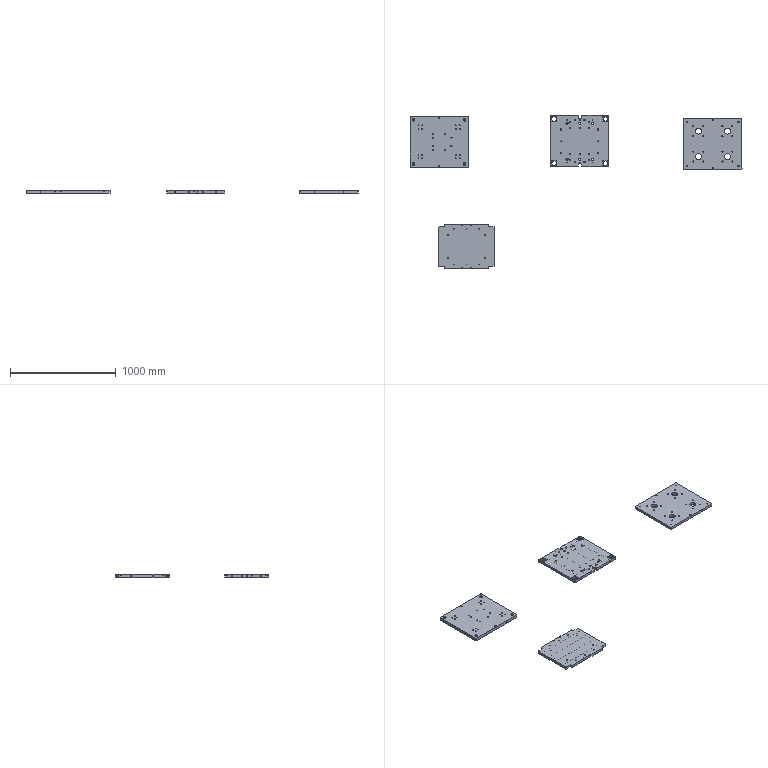NC program | Mastercam | posted with a generic post | part box 3140 x 1452 x 30 mm
Lines 2204 to 3077 of 22248:
N2200 T16 M6
N2210 G0 G90 G17 G54 X-237.285 Y214.441 A0. S6000 M3
N2220 G43 H16 Z50. M8
N2230 Z3.3
N2240 G1 Z.5 F600.
N2250 G3 X-242. Y216.2 Z.437 I-4.715 J-5.441 F3000.
N2260 X-249.2 Y209. Z.299 I0. J-7.2
N2270 X-242. Y201.8 Z.161 I7.2 J0.
N2280 X-234.8 Y209. Z.023 I0. J7.2
N2290 X-242. Y216.2 Z-.116 I-7.2 J0.
N2300 X-249.2 Y209. Z-.254 I0. J-7.2
N2310 X-242. Y201.8 Z-.392 I7.2 J0.
N2320 X-234.8 Y209. Z-.53 I0. J7.2
N2330 X-242. Y216.2 Z-.668 I-7.2 J0.
N2340 X-249.2 Y209. Z-.806 I0. J-7.2
N2350 X-242. Y201.8 Z-.945 I7.2 J0.
N2360 X-234.8 Y209. Z-1.083 I0. J7.2
N2370 X-242. Y216.2 Z-1.221 I-7.2 J0.
N2380 X-249.2 Y209. Z-1.359 I0. J-7.2
N2390 X-242. Y201.8 Z-1.497 I7.2 J0.
N2400 X-234.8 Y209. Z-1.636 I0. J7.2
N2410 X-242. Y216.2 Z-1.774 I-7.2 J0.
N2420 X-249.2 Y209. Z-1.912 I0. J-7.2
N2430 X-242. Y201.8 Z-2.05 I7.2 J0.
N2440 X-234.8 Y209. Z-2.188 I0. J7.2
N2450 X-242. Y216.2 Z-2.326 I-7.2 J0.
N2460 X-249.2 Y209. Z-2.465 I0. J-7.2
N2470 X-242. Y201.8 Z-2.603 I7.2 J0.
N2480 X-234.8 Y209. Z-2.741 I0. J7.2
N2490 X-242. Y216.2 Z-2.879 I-7.2 J0.
N2500 X-249.2 Y209. Z-3.017 I0. J-7.2
N2510 X-242. Y201.8 Z-3.156 I7.2 J0.
N2520 X-234.8 Y209. Z-3.294 I0. J7.2
N2530 X-242. Y216.2 Z-3.432 I-7.2 J0.
N2540 X-249.2 Y209. Z-3.57 I0. J-7.2
N2550 X-242. Y201.8 Z-3.708 I7.2 J0.
N2560 X-234.8 Y209. Z-3.846 I0. J7.2
N2570 X-242. Y216.2 Z-3.985 I-7.2 J0.
N2580 X-249.2 Y209. Z-4.123 I0. J-7.2
N2590 X-242. Y201.8 Z-4.261 I7.2 J0.
N2600 X-234.8 Y209. Z-4.399 I0. J7.2
N2610 X-242. Y216.2 Z-4.537 I-7.2 J0.
N2620 X-249.2 Y209. Z-4.676 I0. J-7.2
N2630 X-242. Y201.8 Z-4.814 I7.2 J0.
N2640 X-234.8 Y209. Z-4.952 I0. J7.2
N2650 X-242. Y216.2 Z-5.09 I-7.2 J0.
N2660 X-249.2 Y209. Z-5.228 I0. J-7.2
N2670 X-242. Y201.8 Z-5.366 I7.2 J0.
N2680 X-234.8 Y209. Z-5.505 I0. J7.2
N2690 X-242. Y216.2 Z-5.643 I-7.2 J0.
N2700 X-249.2 Y209. Z-5.781 I0. J-7.2
N2710 X-242. Y201.8 Z-5.919 I7.2 J0.
N2720 X-234.8 Y209. Z-6.057 I0. J7.2
N2730 X-242. Y216.2 Z-6.196 I-7.2 J0.
N2740 X-249.2 Y209. Z-6.334 I0. J-7.2
N2750 X-242. Y201.8 Z-6.472 I7.2 J0.
N2760 X-234.8 Y209. Z-6.61 I0. J7.2
N2770 X-242. Y216.2 Z-6.748 I-7.2 J0.
N2780 X-249.2 Y209. Z-6.886 I0. J-7.2
N2790 X-242. Y201.8 Z-7.025 I7.2 J0.
N2800 X-234.8 Y209. Z-7.163 I0. J7.2
N2810 X-242. Y216.2 Z-7.301 I-7.2 J0.
N2820 X-249.2 Y209. Z-7.439 I0. J-7.2
N2830 X-242. Y201.8 Z-7.577 I7.2 J0.
N2840 X-234.8 Y209. Z-7.716 I0. J7.2
N2850 X-242. Y216.2 Z-7.854 I-7.2 J0.
N2860 X-249.2 Y209. Z-7.992 I0. J-7.2
N2870 X-242. Y201.8 Z-8.13 I7.2 J0.
N2880 X-234.8 Y209. Z-8.268 I0. J7.2
N2890 X-242. Y216.2 Z-8.406 I-7.2 J0.
N2900 X-249.2 Y209. Z-8.545 I0. J-7.2
N2910 X-242. Y201.8 Z-8.683 I7.2 J0.
N2920 X-234.8 Y209. Z-8.821 I0. J7.2
N2930 X-242. Y216.2 Z-8.959 I-7.2 J0.
N2940 X-249.2 Y209. Z-9.097 I0. J-7.2
N2950 X-242. Y201.8 Z-9.236 I7.2 J0.
N2960 X-234.8 Y209. Z-9.374 I0. J7.2
N2970 X-242. Y216.2 Z-9.512 I-7.2 J0.
N2980 X-249.2 Y209. Z-9.65 I0. J-7.2
N2990 X-242. Y201.8 Z-9.788 I7.2 J0.
N3000 X-234.8 Y209. Z-9.926 I0. J7.2
N3010 X-242. Y216.2 Z-10.065 I-7.2 J0.
N3020 X-249.2 Y209. Z-10.203 I0. J-7.2
N3030 X-242. Y201.8 Z-10.341 I7.2 J0.
N3040 X-234.8 Y209. Z-10.479 I0. J7.2
N3050 X-242. Y216.2 Z-10.617 I-7.2 J0.
N3060 X-249.2 Y209. Z-10.756 I0. J-7.2
N3070 X-242. Y201.8 Z-10.894 I7.2 J0.
N3080 X-234.8 Y209. Z-11.032 I0. J7.2
N3090 X-242. Y216.2 Z-11.17 I-7.2 J0.
N3100 X-249.2 Y209. Z-11.308 I0. J-7.2
N3110 X-242. Y201.8 Z-11.446 I7.2 J0.
N3120 X-234.8 Y209. Z-11.585 I0. J7.2
N3130 X-242. Y216.2 Z-11.723 I-7.2 J0.
N3140 X-249.2 Y209. Z-11.861 I0. J-7.2
N3150 X-242. Y201.8 Z-11.999 I7.2 J0.
N3160 X-234.8 Y209. Z-12.137 I0. J7.2
N3170 X-242. Y216.2 Z-12.275 I-7.2 J0.
N3180 X-249.2 Y209. Z-12.414 I0. J-7.2
N3190 X-242. Y201.8 Z-12.552 I7.2 J0.
N3200 X-234.8 Y209. Z-12.69 I0. J7.2
N3210 X-242. Y216.2 Z-12.828 I-7.2 J0.
N3220 X-249.2 Y209. Z-12.966 I0. J-7.2
N3230 X-242. Y201.8 Z-13.105 I7.2 J0.
N3240 X-234.8 Y209. Z-13.243 I0. J7.2
N3250 X-242. Y216.2 Z-13.381 I-7.2 J0.
N3260 X-249.2 Y209. Z-13.519 I0. J-7.2
N3270 X-242. Y201.8 Z-13.657 I7.2 J0.
N3280 X-234.8 Y209. Z-13.795 I0. J7.2
N3290 X-242. Y216.2 Z-13.934 I-7.2 J0.
N3300 X-249.2 Y209. Z-14.072 I0. J-7.2
N3310 X-242. Y201.8 Z-14.21 I7.2 J0.
N3320 X-234.8 Y209. Z-14.348 I0. J7.2
N3330 X-242. Y216.2 Z-14.486 I-7.2 J0.
N3340 X-249.2 Y209. Z-14.625 I0. J-7.2
N3350 X-242. Y201.8 Z-14.763 I7.2 J0.
N3360 X-234.8 Y209. Z-14.901 I0. J7.2
N3370 X-242. Y216.2 Z-15.039 I-7.2 J0.
N3380 X-249.2 Y209. Z-15.177 I0. J-7.2
N3390 X-242. Y201.8 Z-15.315 I7.2 J0.
N3400 X-234.8 Y209. Z-15.454 I0. J7.2
N3410 X-242. Y216.2 Z-15.592 I-7.2 J0.
N3420 X-249.2 Y209. Z-15.73 I0. J-7.2
N3430 X-242. Y201.8 Z-15.868 I7.2 J0.
N3440 X-234.8 Y209. Z-16.006 I0. J7.2
N3450 X-242. Y216.2 Z-16.145 I-7.2 J0.
N3460 X-249.2 Y209. Z-16.283 I0. J-7.2
N3470 X-242. Y201.8 Z-16.421 I7.2 J0.
N3480 X-234.8 Y209. Z-16.559 I0. J7.2
N3490 X-242. Y216.2 Z-16.697 I-7.2 J0.
N3500 X-249.2 Y209. Z-16.835 I0. J-7.2
N3510 X-242. Y201.8 Z-16.974 I7.2 J0.
N3520 X-234.8 Y209. Z-17.112 I0. J7.2
N3530 X-242. Y216.2 Z-17.25 I-7.2 J0.
N3540 X-249.2 Y209. Z-17.388 I0. J-7.2
N3550 X-242. Y201.8 Z-17.526 I7.2 J0.
N3560 X-234.8 Y209. Z-17.665 I0. J7.2
N3570 X-242. Y216.2 Z-17.803 I-7.2 J0.
N3580 X-249.2 Y209. Z-17.941 I0. J-7.2
N3590 X-242. Y201.8 Z-18.079 I7.2 J0.
N3600 X-234.8 Y209. Z-18.217 I0. J7.2
N3610 X-242. Y216.2 Z-18.355 I-7.2 J0.
N3620 X-249.2 Y209. Z-18.494 I0. J-7.2
N3630 X-242. Y201.8 Z-18.632 I7.2 J0.
N3640 X-234.8 Y209. Z-18.77 I0. J7.2
N3650 X-242. Y216.2 Z-18.908 I-7.2 J0.
N3660 X-249.2 Y209. Z-19.046 I0. J-7.2
N3670 X-242. Y201.8 Z-19.185 I7.2 J0.
N3680 X-234.8 Y209. Z-19.323 I0. J7.2
N3690 X-242. Y216.2 Z-19.461 I-7.2 J0.
N3700 X-249.2 Y209. Z-19.599 I0. J-7.2
N3710 X-242. Y201.8 Z-19.737 I7.2 J0.
N3720 X-234.8 Y209. Z-19.875 I0. J7.2
N3730 X-242. Y216.2 Z-20.014 I-7.2 J0.
N3740 X-249.2 Y209. Z-20.152 I0. J-7.2
N3750 X-242. Y201.8 Z-20.29 I7.2 J0.
N3760 X-234.8 Y209. Z-20.428 I0. J7.2
N3770 X-242. Y216.2 Z-20.566 I-7.2 J0.
N3780 X-249.2 Y209. Z-20.705 I0. J-7.2
N3790 X-242. Y201.8 Z-20.843 I7.2 J0.
N3800 X-234.8 Y209. Z-20.981 I0. J7.2
N3810 X-242. Y216.2 Z-21.119 I-7.2 J0.
N3820 X-249.2 Y209. Z-21.257 I0. J-7.2
N3830 X-242. Y201.8 Z-21.395 I7.2 J0.
N3840 X-234.8 Y209. Z-21.534 I0. J7.2
N3850 X-242. Y216.2 Z-21.672 I-7.2 J0.
N3860 X-249.2 Y209. Z-21.81 I0. J-7.2
N3870 X-242. Y201.8 Z-21.948 I7.2 J0.
N3880 X-234.8 Y209. Z-22.086 I0. J7.2
N3890 X-242. Y216.2 Z-22.225 I-7.2 J0.
N3900 X-249.2 Y209. Z-22.363 I0. J-7.2
N3910 X-242. Y201.8 Z-22.501 I7.2 J0.
N3920 X-234.8 Y209. Z-22.639 I0. J7.2
N3930 X-242. Y216.2 Z-22.777 I-7.2 J0.
N3940 X-249.2 Y209. Z-22.915 I0. J-7.2
N3950 X-242. Y201.8 Z-23.054 I7.2 J0.
N3960 X-234.8 Y209. Z-23.192 I0. J7.2
N3970 X-242. Y216.2 Z-23.33 I-7.2 J0.
N3980 X-249.2 Y209. Z-23.468 I0. J-7.2
N3990 X-242. Y201.8 Z-23.606 I7.2 J0.
N4000 X-234.8 Y209. Z-23.745 I0. J7.2
N4010 X-242. Y216.2 Z-23.883 I-7.2 J0.
N4020 X-249.2 Y209. Z-24.021 I0. J-7.2
N4030 X-242. Y201.8 Z-24.159 I7.2 J0.
N4040 X-234.8 Y209. Z-24.297 I0. J7.2
N4050 X-242. Y216.2 Z-24.435 I-7.2 J0.
N4060 X-249.2 Y209. Z-24.574 I0. J-7.2
N4070 X-242. Y201.8 Z-24.712 I7.2 J0.
N4080 X-234.8 Y209. Z-24.85 I0. J7.2
N4090 X-242. Y216.2 I-7.2 J0.
N4100 X-249.2 Y209. I0. J-7.2
N4110 X-242. Y201.8 I7.2 J0.
N4120 X-234.8 Y209. I0. J7.2
N4130 G1 X-234.788 Y209.214
N4140 X-234.783 Y209.401
N4150 X-234.789 Y209.629
N4160 X-234.807 Y209.881
N4170 X-234.839 Y210.147
N4180 X-234.883 Y210.42
N4190 X-234.94 Y210.697
N4200 X-235.01 Y210.975
N4210 X-235.091 Y211.252
N4220 X-235.184 Y211.527
N4230 X-235.289 Y211.798
N4240 X-235.404 Y212.066
N4250 X-235.531 Y212.329
N4260 X-235.668 Y212.587
N4270 X-235.815 Y212.839
N4280 X-235.973 Y213.085
N4290 X-236.14 Y213.325
N4300 X-236.317 Y213.558
N4310 X-236.503 Y213.783
N4320 X-236.698 Y214.001
N4330 X-236.901 Y214.211
N4340 X-237.113 Y214.412
N4350 X-237.332 Y214.605
N4360 X-237.559 Y214.789
N4370 X-237.793 Y214.964
N4380 X-238.034 Y215.129
N4390 X-238.281 Y215.284
N4400 X-238.535 Y215.429
N4410 X-238.793 Y215.564
N4420 X-239.057 Y215.689
N4430 X-239.326 Y215.803
N4440 X-239.599 Y215.906
N4450 X-239.876 Y215.998
N4460 X-240.157 Y216.079
N4470 X-240.44 Y216.149
N4480 X-240.726 Y216.207
N4490 X-241.014 Y216.254
N4500 X-241.303 Y216.289
N4510 X-241.594 Y216.313
N4520 X-241.886 Y216.325
N4530 X-242.178 Y216.326
N4540 X-242.469 Y216.315
N4550 X-242.76 Y216.292
N4560 X-243.05 Y216.258
N4570 X-243.338 Y216.213
N4580 X-243.624 Y216.156
N4590 X-243.908 Y216.087
N4600 X-244.188 Y216.008
N4610 X-244.466 Y215.917
N4620 X-244.739 Y215.815
N4630 X-245.009 Y215.703
N4640 X-245.273 Y215.58
N4650 X-245.533 Y215.446
N4660 X-245.787 Y215.303
N4670 X-246.035 Y215.149
N4680 X-246.277 Y214.986
N4690 X-246.512 Y214.813
N4700 X-246.74 Y214.631
N4710 X-246.961 Y214.44
N4720 X-247.174 Y214.24
N4730 X-247.379 Y214.032
N4740 X-247.576 Y213.816
N4750 X-247.763 Y213.593
N4760 X-247.942 Y213.362
N4770 X-248.112 Y213.125
N4780 X-248.272 Y212.88
N4790 X-248.423 Y212.63
N4800 X-248.563 Y212.374
N4810 X-248.693 Y212.112
N4820 X-248.813 Y211.846
N4830 X-248.922 Y211.575
N4840 X-249.02 Y211.299
N4850 X-249.107 Y211.02
N4860 X-249.183 Y210.738
N4870 X-249.248 Y210.453
N4880 X-249.302 Y210.166
N4890 X-249.344 Y209.877
N4900 X-249.375 Y209.586
N4910 X-249.394 Y209.294
N4920 X-249.402 Y209.002
N4930 X-249.398 Y208.709
N4940 X-249.383 Y208.417
N4950 X-249.356 Y208.126
N4960 X-249.318 Y207.836
N4970 X-249.268 Y207.547
N4980 X-249.207 Y207.261
N4990 X-249.135 Y206.978
N5000 X-249.051 Y206.697
N5010 X-248.956 Y206.42
N5020 X-248.851 Y206.147
N5030 X-248.735 Y205.878
N5040 X-248.608 Y205.614
N5050 X-248.471 Y205.355
N5060 X-248.324 Y205.102
N5070 X-248.167 Y204.854
N5080 X-248. Y204.613
N5090 X-247.824 Y204.379
N5100 X-247.639 Y204.152
N5110 X-247.445 Y203.932
N5120 X-247.243 Y203.72
N5130 X-247.032 Y203.516
N5140 X-246.813 Y203.321
N5150 X-246.587 Y203.134
N5160 X-246.354 Y202.956
N5170 X-246.113 Y202.788
N5180 X-245.866 Y202.629
N5190 X-245.614 Y202.48
N5200 X-245.355 Y202.341
N5210 X-245.091 Y202.213
N5220 X-244.822 Y202.094
N5230 X-244.549 Y201.987
N5240 X-244.272 Y201.89
N5250 X-243.991 Y201.804
N5260 X-243.707 Y201.73
N5270 X-243.42 Y201.666
N5280 X-243.13 Y201.614
N5290 X-242.839 Y201.574
N5300 X-242.547 Y201.544
N5310 X-242.253 Y201.527
N5320 X-241.959 Y201.521
N5330 X-241.665 Y201.526
N5340 X-241.371 Y201.543
N5350 X-241.078 Y201.572
N5360 X-240.787 Y201.612
N5370 X-240.497 Y201.663
N5380 X-240.209 Y201.726
N5390 X-239.924 Y201.8
N5400 X-239.643 Y201.885
N5410 X-239.364 Y201.982
N5420 X-239.09 Y202.089
N5430 X-238.82 Y202.207
N5440 X-238.555 Y202.335
N5450 X-238.294 Y202.474
N5460 X-238.04 Y202.623
N5470 X-237.792 Y202.781
N5480 X-237.55 Y202.95
N5490 X-237.314 Y203.128
N5500 X-237.086 Y203.315
N5510 X-236.865 Y203.51
N5520 X-236.652 Y203.715
N5530 X-236.448 Y203.927
N5540 X-236.251 Y204.148
N5550 X-236.064 Y204.376
N5560 X-235.885 Y204.611
N5570 X-235.716 Y204.854
N5580 X-235.557 Y205.102
N5590 X-235.407 Y205.357
N5600 X-235.268 Y205.618
N5610 X-235.138 Y205.884
N5620 X-235.02 Y206.156
N5630 X-234.912 Y206.434
N5640 X-234.815 Y206.716
N5650 X-234.729 Y207.002
N5660 X-234.654 Y207.295
N5670 X-234.582 Y207.627
N5680 X-234.525 Y207.941
N5690 X-234.482 Y208.246
N5700 X-234.452 Y208.546
N5710 X-234.434 Y208.843
N5720 X-234.427 Y209.139
N5730 X-234.433 Y209.434
N5740 X-234.451 Y209.728
N5750 X-234.48 Y210.022
N5760 X-234.521 Y210.315
N5770 X-234.575 Y210.607
N5780 X-234.64 Y210.897
N5790 X-234.716 Y211.184
N5800 X-234.804 Y211.469
N5810 X-234.904 Y211.75
N5820 X-235.015 Y212.028
N5830 X-235.137 Y212.302
N5840 X-235.27 Y212.57
N5850 X-235.414 Y212.834
N5860 X-235.568 Y213.092
N5870 X-235.733 Y213.344
N5880 X-235.907 Y213.589
N5890 X-236.092 Y213.827
N5900 X-236.285 Y214.058
N5910 X-236.488 Y214.282
N5920 X-236.7 Y214.497
N5930 X-236.92 Y214.703
N5940 X-237.148 Y214.901
N5950 X-237.384 Y215.09
N5960 X-237.627 Y215.269
N5970 X-237.877 Y215.439
N5980 X-238.134 Y215.599
N5990 X-238.397 Y215.748
N6000 X-238.666 Y215.887
N6010 X-238.94 Y216.015
N6020 X-239.219 Y216.133
N6030 X-239.503 Y216.239
N6040 X-239.791 Y216.334
N6050 X-240.082 Y216.417
N6060 X-240.376 Y216.489
N6070 X-240.673 Y216.549
N6080 X-240.972 Y216.598
N6090 X-241.273 Y216.634
N6100 X-241.575 Y216.659
N6110 X-241.878 Y216.672
N6120 X-242.182
N6130 X-242.485 Y216.661
N6140 X-242.787 Y216.638
N6150 X-243.089 Y216.603
N6160 X-243.389 Y216.556
N6170 X-243.686 Y216.497
N6180 X-243.982 Y216.426
N6190 X-244.274 Y216.344
N6200 X-244.563 Y216.25
N6210 X-244.848 Y216.145
N6220 X-245.128 Y216.029
N6230 X-245.404 Y215.902
N6240 X-245.675 Y215.764
N6250 X-245.94 Y215.615
N6260 X-246.199 Y215.456
N6270 X-246.452 Y215.287
N6280 X-246.697 Y215.108
N6290 X-246.936 Y214.919
N6300 X-247.167 Y214.721
N6310 X-247.39 Y214.515
N6320 X-247.604 Y214.299
N6330 X-247.811 Y214.075
N6340 X-248.008 Y213.843
N6350 X-248.195 Y213.604
N6360 X-248.374 Y213.357
N6370 X-248.542 Y213.104
N6380 X-248.7 Y212.844
N6390 X-248.848 Y212.578
N6400 X-248.986 Y212.306
N6410 X-249.112 Y212.029
N6420 X-249.228 Y211.748
N6430 X-249.332 Y211.462
N6440 X-249.425 Y211.172
N6450 X-249.507 Y210.879
N6460 X-249.577 Y210.582
N6470 X-249.635 Y210.283
N6480 X-249.681 Y209.982
N6490 X-249.716 Y209.68
N6500 X-249.739 Y209.376
N6510 X-249.75 Y209.072
N6520 X-249.748 Y208.767
N6530 X-249.735 Y208.463
N6540 X-249.71 Y208.159
N6550 X-249.673 Y207.857
N6560 X-249.624 Y207.556
N6570 X-249.564 Y207.258
N6580 X-249.491 Y206.962
N6590 X-249.407 Y206.669
N6600 X-249.312 Y206.379
N6610 X-249.205 Y206.094
N6620 X-249.088 Y205.813
N6630 X-248.959 Y205.536
N6640 X-248.82 Y205.265
N6650 X-248.67 Y205.
N6660 X-248.51 Y204.741
N6670 X-248.339 Y204.488
N6680 X-248.159 Y204.242
N6690 X-247.97 Y204.003
N6700 X-247.771 Y203.772
N6710 X-247.563 Y203.548
N6720 X-247.347 Y203.333
N6730 X-247.122 Y203.127
N6740 X-246.89 Y202.93
N6750 X-246.65 Y202.741
N6760 X-246.403 Y202.563
N6770 X-246.149 Y202.394
N6780 X-245.888 Y202.235
N6790 X-245.622 Y202.087
N6800 X-245.35 Y201.948
N6810 X-245.073 Y201.821
N6820 X-244.79 Y201.705
N6830 X-244.504 Y201.6
N6840 X-244.214 Y201.505
N6850 X-243.92 Y201.423
N6860 X-243.623 Y201.352
N6870 X-243.324 Y201.292
N6880 X-243.022 Y201.245
N6890 X-242.719 Y201.209
N6900 X-242.415 Y201.185
N6910 X-242.11 Y201.172
N6920 X-241.804
N6930 X-241.499 Y201.184
N6940 X-241.195 Y201.207
N6950 X-240.891 Y201.242
N6960 X-240.589 Y201.29
N6970 X-240.29 Y201.349
N6980 X-239.992 Y201.419
N6990 X-239.698 Y201.501
N7000 X-239.407 Y201.595
N7010 X-239.12 Y201.699
N7020 X-238.837 Y201.815
N7030 X-238.559 Y201.942
N7040 X-238.286 Y202.079
N7050 X-238.019 Y202.227
N7060 X-237.757 Y202.386
N7070 X-237.502 Y202.554
N7080 X-237.253 Y202.732
N7090 X-237.012 Y202.92
N7100 X-236.778 Y203.117
N7110 X-236.552 Y203.323
N7120 X-236.334 Y203.538
N7130 X-236.124 Y203.761
N7140 X-235.924 Y203.992
N7150 X-235.732 Y204.23
N7160 X-235.551 Y204.476
N7170 X-235.379 Y204.728
N7180 X-235.217 Y204.986
N7190 X-235.065 Y205.251
N7200 X-234.924 Y205.522
N7210 X-234.793 Y205.799
N7220 X-234.67 Y206.087
N7230 X-234.558 Y206.381
N7240 X-234.456 Y206.679
N7250 X-234.367 Y206.98
N7260 X-234.289 Y207.283
N7270 X-234.223 Y207.587
N7280 X-234.169 Y207.892
N7290 X-234.127 Y208.198
N7300 X-234.098 Y208.505
N7310 X-234.08 Y208.812
N7320 X-234.074 Y209.119
N7330 X-234.08 Y209.426
N7340 X-234.098 Y209.732
N7350 X-234.128 Y210.037
N7360 X-234.171 Y210.34
N7370 X-234.224 Y210.642
N7380 X-234.29 Y210.942
N7390 X-234.368 Y211.238
N7400 X-234.456 Y211.532
N7410 X-234.557 Y211.822
N7420 X-234.668 Y212.108
N7430 X-234.791 Y212.389
N7440 X-234.925 Y212.666
N7450 X-235.069 Y212.937
N7460 X-235.224 Y213.202
N7470 X-235.389 Y213.462
N7480 X-235.563 Y213.715
N7490 X-235.748 Y213.961
N7500 X-235.942 Y214.199
N7510 X-236.145 Y214.43
N7520 X-236.357 Y214.653
N7530 X-236.578 Y214.868
N7540 X-236.806 Y215.074
N7550 X-237.043 Y215.271
N7560 X-237.286 Y215.459
N7570 X-237.537 Y215.637
N7580 X-237.795 Y215.806
N7590 X-238.059 Y215.964
N7600 X-238.33 Y216.113
N7610 X-238.606 Y216.251
N7620 X-238.887 Y216.378
N7630 X-239.173 Y216.494
N7640 X-239.464 Y216.6
N7650 X-239.758 Y216.694
N7660 X-240.056 Y216.776
N7670 X-240.357 Y216.847
N7680 X-240.661 Y216.907
N7690 X-240.967 Y216.955
N7700 X-241.275 Y216.99
N7710 X-241.584 Y217.014
N7720 X-241.894 Y217.026
N7730 X-242.204
N7740 X-242.514 Y217.014
N7750 X-242.823 Y216.991
N7760 X-243.132 Y216.955
N7770 X-243.438 Y216.907
N7780 X-243.743 Y216.847
N7790 X-244.045 Y216.776
N7800 X-244.345 Y216.693
N7810 X-244.64 Y216.599
N7820 X-244.932 Y216.493
N7830 X-245.219 Y216.376
N7840 X-245.502 Y216.249
N7850 X-245.779 Y216.11
N7860 X-246.051 Y215.961
N7870 X-246.317 Y215.802
N7880 X-246.576 Y215.632
N7890 X-246.829 Y215.453
N7900 X-247.074 Y215.264
N7910 X-247.312 Y215.066
N7920 X-247.543 Y214.859
N7930 X-247.765 Y214.644
N7940 X-247.978 Y214.42
N7950 X-248.183 Y214.188
N7960 X-248.379 Y213.948
N7970 X-248.566 Y213.701
N7980 X-248.743 Y213.447
N7990 X-248.91 Y213.186
N8000 X-249.067 Y212.919
N8010 X-249.214 Y212.646
N8020 X-249.35 Y212.367
N8030 X-249.476 Y212.084
N8040 X-249.59 Y211.795
N8050 X-249.694 Y211.502
N8060 X-249.786 Y211.205
N8070 X-249.867 Y210.905
N8080 X-249.936 Y210.602
N8090 X-249.994 Y210.296
N8100 X-250.04 Y209.988
N8110 X-250.074 Y209.679
N8120 X-250.096 Y209.368
N8130 X-250.106 Y209.057
N8140 X-250.104 Y208.745
N8150 X-250.09 Y208.434
N8160 X-250.064 Y208.123
N8170 X-250.027 Y207.814
N8180 X-249.977 Y207.506
N8190 X-249.916 Y207.2
N8200 X-249.843 Y206.897
N8210 X-249.758 Y206.596
N8220 X-249.662 Y206.3
N8230 X-249.554 Y206.007
N8240 X-249.436 Y205.719
N8250 X-249.306 Y205.435
N8260 X-249.166 Y205.157
N8270 X-249.016 Y204.885
N8280 X-248.855 Y204.618
N8290 X-248.683 Y204.358
N8300 X-248.503 Y204.105
N8310 X-248.312 Y203.858
N8320 X-248.113 Y203.619
N8330 X-247.904 Y203.389
N8340 X-247.687 Y203.166
N8350 X-247.461 Y202.951
N8360 X-247.227 Y202.746
N8370 X-246.986 Y202.549
N8380 X-246.738 Y202.362
N8390 X-246.482 Y202.185
N8400 X-246.22 Y202.017
N8410 X-245.952 Y201.86
N8420 X-245.678 Y201.712
N8430 X-245.398 Y201.576
N8440 X-245.113 Y201.45
N8450 X-244.823 Y201.335
N8460 X-244.529 Y201.231
N8470 X-244.231 Y201.138
N8480 X-243.93 Y201.056
N8490 X-243.626 Y200.987
N8500 X-243.319 Y200.928
N8510 X-243.01 Y200.882
N8520 X-242.699 Y200.847
N8530 X-242.388 Y200.825
N8540 X-242.075 Y200.814
N8550 X-241.762 Y200.815
N8560 X-241.45 Y200.828
N8570 X-241.137 Y200.853
N8580 X-240.827 Y200.89
N8590 X-240.517 Y200.939
N8600 X-240.21 Y200.999
N8610 X-239.905 Y201.072
N8620 X-239.603 Y201.156
N8630 X-239.304 Y201.251
N8640 X-239.01 Y201.358
N8650 X-238.719 Y201.476
N8660 X-238.433 Y201.605
N8670 X-238.153 Y201.745
N8680 X-237.878 Y201.895
N8690 X-237.609 Y202.056
N8700 X-237.346 Y202.226
N8710 X-237.09 Y202.407
N8720 X-236.841 Y202.597
N8730 X-236.6 Y202.797
N8740 X-236.367 Y203.005
N8750 X-236.141 Y203.222
N8760 X-235.925 Y203.448
N8770 X-235.717 Y203.681
N8780 X-235.519 Y203.922
N8790 X-235.33 Y204.17
N8800 X-235.15 Y204.425
N8810 X-234.979 Y204.689
N8820 X-234.818 Y204.959
N8830 X-234.667 Y205.236
N8840 X-234.526 Y205.519
N8850 X-234.395 Y205.807
N8860 X-234.276 Y206.1
N8870 X-234.168 Y206.396
N8880 X-234.071 Y206.697
N8890 X-233.985 Y207.
N8900 X-233.911 Y207.307
N8910 X-233.848 Y207.615
N8920 X-233.798 Y207.925
N8930 X-233.759 Y208.237
N8940 X-233.732 Y208.55
N8950 X-233.717 Y208.863
N8960 X-233.714 Y209.177
N8970 X-233.723 Y209.491
N8980 X-233.743 Y209.804
N8990 X-233.776 Y210.116
N9000 X-233.821 Y210.426
N9010 X-233.877 Y210.735
N9020 X-233.945 Y211.041
N9030 X-234.025 Y211.345
N9040 X-234.116 Y211.645
N9050 X-234.219 Y211.942
N9060 X-234.333 Y212.235
N9070 X-234.458 Y212.524
N9080 X-234.594 Y212.808
N9090 X-234.741 Y213.086
N9100 X-234.898 Y213.359
N9110 X-235.065 Y213.625
N9120 X-235.243 Y213.885
N9130 X-235.43 Y214.138
N9140 X-235.627 Y214.384
N9150 X-235.833 Y214.622
N9160 X-236.048 Y214.852
N9170 X-236.271 Y215.074
N9180 X-236.503 Y215.287
N9190 X-236.742 Y215.492
N9200 X-236.989 Y215.687
N9210 X-237.243 Y215.873
N9220 X-237.504 Y216.049
N9230 X-237.772 Y216.215
N9240 X-238.045 Y216.37
N9250 X-238.325 Y216.516
N9260 X-238.609 Y216.651
N9270 X-238.899 Y216.774
N9280 X-239.192 Y216.887
N9290 X-239.49 Y216.989
N9300 X-239.792 Y217.08
N9310 X-240.097 Y217.159
N9320 X-240.404 Y217.227
N9330 X-240.715 Y217.283
N9340 X-241.027 Y217.327
N9350 X-241.341 Y217.36
N9360 X-241.656 Y217.381
N9370 X-241.972 Y217.39
N9380 X-242.288 Y217.387
N9390 X-242.604 Y217.372
N9400 X-242.919 Y217.345
N9410 X-243.233 Y217.306
N9420 X-243.545 Y217.256
N9430 X-243.856 Y217.194
N9440 X-244.164 Y217.12
N9450 X-244.469 Y217.034
N9460 X-244.771 Y216.937
N9470 X-245.069 Y216.829
N9480 X-245.362 Y216.71
N9490 X-245.651 Y216.579
N9500 X-245.935 Y216.438
N9510 X-246.214 Y216.286
N9520 X-246.487 Y216.123
N9530 X-246.753 Y215.951
N9540 X-247.012 Y215.768
N9550 X-247.265 Y215.576
N9560 X-247.51 Y215.375
N9570 X-247.747 Y215.165
N9580 X-247.976 Y214.946
N9590 X-248.197 Y214.718
N9600 X-248.409 Y214.483
N9610 X-248.612 Y214.239
N9620 X-248.805 Y213.989
N9630 X-248.989 Y213.731
N9640 X-249.163 Y213.466
N9650 X-249.327 Y213.195
N9660 X-249.481 Y212.919
N9670 X-249.625 Y212.636
N9680 X-249.757 Y212.349
N9690 X-249.879 Y212.057
N9700 X-249.99 Y211.76
N9710 X-250.089 Y211.46
N9720 X-250.178 Y211.156
N9730 X-250.254 Y210.849
N9740 X-250.32 Y210.54
N9750 X-250.373 Y210.228
N9760 X-250.415 Y209.914
N9770 X-250.446 Y209.598
N9780 X-250.464 Y209.282
N9790 X-250.471 Y208.964
N9800 X-250.465 Y208.647
N9810 X-250.448 Y208.33
N9820 X-250.419 Y208.014
N9830 X-250.378 Y207.699
N9840 X-250.325 Y207.385
N9850 X-250.261 Y207.074
N9860 X-250.185 Y206.765
N9870 X-250.097 Y206.459
N9880 X-249.998 Y206.157
N9890 X-249.887 Y205.858
N9900 X-249.766 Y205.564
N9910 X-249.633 Y205.274
N9920 X-249.49 Y204.99
N9930 X-249.336 Y204.711
N9940 X-249.172 Y204.438
N9950 X-248.997 Y204.171
N9960 X-248.813 Y203.911
N9970 X-248.619 Y203.658
N9980 X-248.416 Y203.412
N9990 X-248.203 Y203.175
N100 X-247.982 Y202.945
N110 X-247.753 Y202.724
N120 X-247.516 Y202.512
N130 X-247.27 Y202.309
N140 X-247.018 Y202.115
N150 X-246.758 Y201.931
N160 X-246.492 Y201.757
N170 X-246.22 Y201.592
N180 X-245.941 Y201.438
N190 X-245.657 Y201.295
N200 X-245.368 Y201.162
N210 X-245.075 Y201.04
N220 X-244.777 Y200.929
N230 X-244.475 Y200.829
N240 X-244.169 Y200.741
N250 X-243.861 Y200.664
N260 X-243.55 Y200.599
N270 X-243.236 Y200.545
N280 X-242.921 Y200.503
N290 X-242.604 Y200.473
N300 X-242.287 Y200.454
N310 X-241.968 Y200.447
N320 X-241.65 Y200.452
N330 X-241.332 Y200.469
N340 X-241.014 Y200.498
N350 X-240.698 Y200.539
N360 X-240.383 Y200.591
N370 X-240.07 Y200.656
N380 X-239.76 Y200.731
N390 X-239.452 Y200.819
N400 X-239.149 Y200.918
N410 X-238.848 Y201.028
N420 X-238.552 Y201.149
N430 X-238.261 Y201.281
N440 X-237.975 Y201.424
N450 X-237.694 Y201.578
N460 X-237.419 Y201.742
N470 X-237.151 Y201.916
N480 X-236.889 Y202.1
N490 X-236.634 Y202.294
N500 X-236.387 Y202.497
N510 X-236.148 Y202.709
N520 X-235.916 Y202.93
N530 X-235.693 Y203.159
N540 X-235.479 Y203.396
N550 X-235.273 Y203.642
N560 X-235.077 Y203.895
N570 X-234.889 Y204.156
N580 X-234.712 Y204.424
N590 X-234.544 Y204.698
N600 X-234.386 Y204.979
N610 X-234.239 Y205.265
N620 X-234.102 Y205.556
N630 X-233.977 Y205.852
N640 X-233.862 Y206.152
N650 X-233.758 Y206.457
N660 X-233.666 Y206.764
N670 X-233.586 Y207.074
N680 X-233.516 Y207.387
N690 X-233.459 Y207.702
N700 X-233.413 Y208.019
N710 X-233.379 Y208.337
N720 X-233.357 Y208.656
N730 X-233.346 Y208.975
N740 X-233.348 Y209.295
N750 X-233.361 Y209.614
N760 X-233.386 Y209.933
N770 X-233.423 Y210.251
N780 X-233.472 Y210.567
N790 X-233.532 Y210.881
N800 X-233.604 Y211.193
N810 X-233.688 Y211.502
N820 X-233.783 Y211.808
N830 X-233.889 Y212.111
N840 X-234.007 Y212.409
N850 X-234.136 Y212.703
N860 X-234.275 Y212.992
N870 X-234.426 Y213.276
N880 X-234.586 Y213.554
N890 X-234.758 Y213.826
N900 X-234.939 Y214.092
N910 X-235.13 Y214.35
N920 X-235.33 Y214.602
N930 X-235.54 Y214.846
N940 X-235.758 Y215.082
N950 X-235.985 Y215.31
N960 X-236.221 Y215.529
N970 X-236.464 Y215.74
N980 X-236.715 Y215.941
N990 X-236.973 Y216.133
N1000 X-237.238 Y216.315
N1010 X-237.51 Y216.487
N1020 X-237.788 Y216.649
N1030 X-238.071 Y216.801